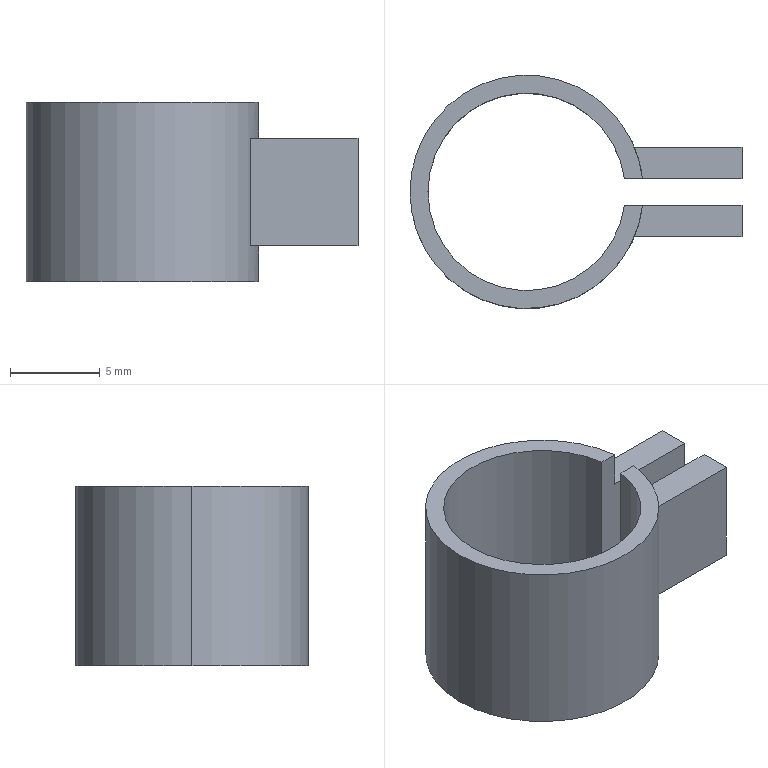Part | SolidWorks | features ICE 2, ExtruThin 1 | 1 solid | 16 faces | box 18.5 x 13 x 10 mm | volume 482.242 mm3 | plane 12 | cylinder 4 | commonest cylinder face diameters 11 x2 13 x2
STEP:
#1=CARTESIAN_POINT('',(5.449,0.75,5.));
#2=VERTEX_POINT('',#1);
#3=CARTESIAN_POINT('',(-5.5,0.,5.));
#4=VERTEX_POINT('',#3);
#5=CARTESIAN_POINT('',(0.,0.,5.));
#6=DIRECTION('',(0.,0.,1.));
#7=DIRECTION('',(1.,0.,0.));
#8=AXIS2_PLACEMENT_3D('',#5,#6,#7);
#9=CIRCLE('',#8,5.5);
#10=EDGE_CURVE('',#2,#4,#9,.T.);
#11=ORIENTED_EDGE('',*,*,#10,.T.);
#12=CARTESIAN_POINT('',(-5.5,0.,-5.));
#13=VERTEX_POINT('',#12);
#14=CARTESIAN_POINT('',(-5.5,0.,5.));
#15=DIRECTION('',(0.,0.,-1.));
#16=VECTOR('',#15,1000.);
#17=LINE('',#14,#16);
#18=EDGE_CURVE('',#4,#13,#17,.T.);
#19=ORIENTED_EDGE('',*,*,#18,.T.);
#20=CARTESIAN_POINT('',(5.449,0.75,-5.));
#21=VERTEX_POINT('',#20);
#22=CARTESIAN_POINT('',(0.,0.,-5.));
#23=DIRECTION('',(0.,0.,1.));
#24=DIRECTION('',(1.,0.,0.));
#25=AXIS2_PLACEMENT_3D('',#22,#23,#24);
#26=CIRCLE('',#25,5.5);
#27=EDGE_CURVE('',#21,#13,#26,.T.);
#28=ORIENTED_EDGE('',*,*,#27,.F.);
#29=CARTESIAN_POINT('',(5.449,0.75,5.));
#30=DIRECTION('',(0.,0.,-1.));
#31=VECTOR('',#30,1000.);
#32=LINE('',#29,#31);
#33=EDGE_CURVE('',#2,#21,#32,.T.);
#34=ORIENTED_EDGE('',*,*,#33,.F.);
#35=EDGE_LOOP('',(#11,#19,#28,#34));
#36=FACE_OUTER_BOUND('',#35,.T.);
#37=CARTESIAN_POINT('',(0.,0.,5.));
#38=DIRECTION('',(0.,0.,-1.));
#39=DIRECTION('',(-1.,0.,0.));
#40=AXIS2_PLACEMENT_3D('',#37,#38,#39);
#41=CYLINDRICAL_SURFACE('',#40,5.5);
#42=ADVANCED_FACE('',(#36),#41,.F.);
#43=CARTESIAN_POINT('',(-6.5,0.,5.));
#44=VERTEX_POINT('',#43);
#45=CARTESIAN_POINT('',(6.457,-0.75,5.));
#46=VERTEX_POINT('',#45);
#47=CARTESIAN_POINT('',(0.,0.,5.));
#48=DIRECTION('',(0.,0.,1.));
#49=DIRECTION('',(1.,0.,0.));
#50=AXIS2_PLACEMENT_3D('',#47,#48,#49);
#51=CIRCLE('',#50,6.5);
#52=EDGE_CURVE('',#44,#46,#51,.T.);
#53=ORIENTED_EDGE('',*,*,#52,.F.);
#54=CARTESIAN_POINT('',(-6.5,0.,-5.));
#55=VERTEX_POINT('',#54);
#56=CARTESIAN_POINT('',(-6.5,0.,5.));
#57=DIRECTION('',(0.,0.,-1.));
#58=VECTOR('',#57,1000.);
#59=LINE('',#56,#58);
#60=EDGE_CURVE('',#44,#55,#59,.T.);
#61=ORIENTED_EDGE('',*,*,#60,.T.);
#62=CARTESIAN_POINT('',(6.457,-0.75,-5.));
#63=VERTEX_POINT('',#62);
#64=CARTESIAN_POINT('',(0.,0.,-5.));
#65=DIRECTION('',(0.,0.,1.));
#66=DIRECTION('',(1.,0.,0.));
#67=AXIS2_PLACEMENT_3D('',#64,#65,#66);
#68=CIRCLE('',#67,6.5);
#69=EDGE_CURVE('',#55,#63,#68,.T.);
#70=ORIENTED_EDGE('',*,*,#69,.T.);
#71=CARTESIAN_POINT('',(6.457,-0.75,-3.));
#72=VERTEX_POINT('',#71);
#73=CARTESIAN_POINT('',(6.457,-0.75,5.));
#74=DIRECTION('',(0.,0.,1.));
#75=VECTOR('',#74,1000.);
#76=LINE('',#73,#75);
#77=EDGE_CURVE('',#63,#72,#76,.T.);
#78=ORIENTED_EDGE('',*,*,#77,.T.);
#79=CARTESIAN_POINT('',(6.,-2.5,-3.));
#80=VERTEX_POINT('',#79);
#81=CARTESIAN_POINT('',(0.,0.,-3.));
#82=DIRECTION('',(0.,0.,1.));
#83=DIRECTION('',(1.,0.,0.));
#84=AXIS2_PLACEMENT_3D('',#81,#82,#83);
#85=CIRCLE('',#84,6.5);
#86=EDGE_CURVE('',#80,#72,#85,.T.);
#87=ORIENTED_EDGE('',*,*,#86,.F.);
#88=CARTESIAN_POINT('',(6.,-2.5,3.));
#89=VERTEX_POINT('',#88);
#90=CARTESIAN_POINT('',(6.,-2.5,3.));
#91=DIRECTION('',(0.,0.,-1.));
#92=VECTOR('',#91,1000.);
#93=LINE('',#90,#92);
#94=EDGE_CURVE('',#89,#80,#93,.T.);
#95=ORIENTED_EDGE('',*,*,#94,.F.);
#96=CARTESIAN_POINT('',(6.457,-0.75,3.));
#97=VERTEX_POINT('',#96);
#98=CARTESIAN_POINT('',(0.,0.,3.));
#99=DIRECTION('',(0.,0.,1.));
#100=DIRECTION('',(1.,0.,0.));
#101=AXIS2_PLACEMENT_3D('',#98,#99,#100);
#102=CIRCLE('',#101,6.5);
#103=EDGE_CURVE('',#89,#97,#102,.T.);
#104=ORIENTED_EDGE('',*,*,#103,.T.);
#105=CARTESIAN_POINT('',(6.457,-0.75,5.));
#106=DIRECTION('',(0.,0.,1.));
#107=VECTOR('',#106,1000.);
#108=LINE('',#105,#107);
#109=EDGE_CURVE('',#97,#46,#108,.T.);
#110=ORIENTED_EDGE('',*,*,#109,.T.);
#111=EDGE_LOOP('',(#53,#61,#70,#78,#87,#95,#104,#110));
#112=FACE_OUTER_BOUND('',#111,.T.);
#113=CARTESIAN_POINT('',(0.,0.,5.));
#114=DIRECTION('',(0.,0.,-1.));
#115=DIRECTION('',(-1.,0.,0.));
#116=AXIS2_PLACEMENT_3D('',#113,#114,#115);
#117=CYLINDRICAL_SURFACE('',#116,6.5);
#118=ADVANCED_FACE('',(#112),#117,.T.);
#119=CARTESIAN_POINT('',(12.,0.75,3.));
#120=VERTEX_POINT('',#119);
#121=CARTESIAN_POINT('',(12.,2.5,3.));
#122=VERTEX_POINT('',#121);
#123=CARTESIAN_POINT('',(12.,2.5,3.));
#124=DIRECTION('',(0.,1.,0.));
#125=VECTOR('',#124,1000.);
#126=LINE('',#123,#125);
#127=EDGE_CURVE('',#120,#122,#126,.T.);
#128=ORIENTED_EDGE('',*,*,#127,.F.);
#129=CARTESIAN_POINT('',(12.,0.75,-3.));
#130=VERTEX_POINT('',#129);
#131=CARTESIAN_POINT('',(12.,0.75,3.));
#132=DIRECTION('',(0.,0.,-1.));
#133=VECTOR('',#132,1000.);
#134=LINE('',#131,#133);
#135=EDGE_CURVE('',#120,#130,#134,.T.);
#136=ORIENTED_EDGE('',*,*,#135,.T.);
#137=CARTESIAN_POINT('',(12.,2.5,-3.));
#138=VERTEX_POINT('',#137);
#139=CARTESIAN_POINT('',(12.,2.5,-3.));
#140=DIRECTION('',(0.,1.,0.));
#141=VECTOR('',#140,1000.);
#142=LINE('',#139,#141);
#143=EDGE_CURVE('',#130,#138,#142,.T.);
#144=ORIENTED_EDGE('',*,*,#143,.T.);
#145=CARTESIAN_POINT('',(12.,2.5,3.));
#146=DIRECTION('',(0.,0.,-1.));
#147=VECTOR('',#146,1000.);
#148=LINE('',#145,#147);
#149=EDGE_CURVE('',#122,#138,#148,.T.);
#150=ORIENTED_EDGE('',*,*,#149,.F.);
#151=EDGE_LOOP('',(#128,#136,#144,#150));
#152=FACE_OUTER_BOUND('',#151,.T.);
#153=CARTESIAN_POINT('',(12.,2.5,3.));
#154=DIRECTION('',(-1.,0.,0.));
#155=DIRECTION('',(0.,0.,1.));
#156=AXIS2_PLACEMENT_3D('',#153,#154,#155);
#157=PLANE('',#156);
#158=ADVANCED_FACE('',(#152),#157,.F.);
#159=CARTESIAN_POINT('',(6.457,0.75,3.));
#160=VERTEX_POINT('',#159);
#161=CARTESIAN_POINT('',(0.,0.75,3.));
#162=DIRECTION('',(-1.,0.,0.));
#163=VECTOR('',#162,1000.);
#164=LINE('',#161,#163);
#165=EDGE_CURVE('',#120,#160,#164,.T.);
#166=ORIENTED_EDGE('',*,*,#165,.F.);
#167=ORIENTED_EDGE('',*,*,#127,.T.);
#168=CARTESIAN_POINT('',(6.,2.5,3.));
#169=VERTEX_POINT('',#168);
#170=CARTESIAN_POINT('',(6.,2.5,3.));
#171=DIRECTION('',(-1.,0.,0.));
#172=VECTOR('',#171,1000.);
#173=LINE('',#170,#172);
#174=EDGE_CURVE('',#122,#169,#173,.T.);
#175=ORIENTED_EDGE('',*,*,#174,.T.);
#176=CARTESIAN_POINT('',(0.,0.,3.));
#177=DIRECTION('',(0.,0.,1.));
#178=DIRECTION('',(1.,0.,0.));
#179=AXIS2_PLACEMENT_3D('',#176,#177,#178);
#180=CIRCLE('',#179,6.5);
#181=EDGE_CURVE('',#160,#169,#180,.T.);
#182=ORIENTED_EDGE('',*,*,#181,.F.);
#183=EDGE_LOOP('',(#166,#167,#175,#182));
#184=FACE_OUTER_BOUND('',#183,.T.);
#185=CARTESIAN_POINT('',(0.,0.,3.));
#186=DIRECTION('',(0.,0.,1.));
#187=DIRECTION('',(1.,0.,0.));
#188=AXIS2_PLACEMENT_3D('',#185,#186,#187);
#189=PLANE('',#188);
#190=ADVANCED_FACE('',(#184),#189,.T.);
#191=ORIENTED_EDGE('',*,*,#143,.F.);
#192=CARTESIAN_POINT('',(6.457,0.75,-3.));
#193=VERTEX_POINT('',#192);
#194=CARTESIAN_POINT('',(0.,0.75,-3.));
#195=DIRECTION('',(-1.,0.,0.));
#196=VECTOR('',#195,1000.);
#197=LINE('',#194,#196);
#198=EDGE_CURVE('',#130,#193,#197,.T.);
#199=ORIENTED_EDGE('',*,*,#198,.T.);
#200=CARTESIAN_POINT('',(6.,2.5,-3.));
#201=VERTEX_POINT('',#200);
#202=CARTESIAN_POINT('',(0.,0.,-3.));
#203=DIRECTION('',(0.,0.,1.));
#204=DIRECTION('',(1.,0.,0.));
#205=AXIS2_PLACEMENT_3D('',#202,#203,#204);
#206=CIRCLE('',#205,6.5);
#207=EDGE_CURVE('',#193,#201,#206,.T.);
#208=ORIENTED_EDGE('',*,*,#207,.T.);
#209=CARTESIAN_POINT('',(6.,2.5,-3.));
#210=DIRECTION('',(-1.,0.,0.));
#211=VECTOR('',#210,1000.);
#212=LINE('',#209,#211);
#213=EDGE_CURVE('',#138,#201,#212,.T.);
#214=ORIENTED_EDGE('',*,*,#213,.F.);
#215=EDGE_LOOP('',(#191,#199,#208,#214));
#216=FACE_OUTER_BOUND('',#215,.T.);
#217=CARTESIAN_POINT('',(0.,0.,-3.));
#218=DIRECTION('',(0.,0.,1.));
#219=DIRECTION('',(1.,0.,0.));
#220=AXIS2_PLACEMENT_3D('',#217,#218,#219);
#221=PLANE('',#220);
#222=ADVANCED_FACE('',(#216),#221,.F.);
#223=CARTESIAN_POINT('',(6.457,0.75,5.));
#224=VERTEX_POINT('',#223);
#225=CARTESIAN_POINT('',(0.,0.75,5.));
#226=DIRECTION('',(-1.,0.,0.));
#227=VECTOR('',#226,1000.);
#228=LINE('',#225,#227);
#229=EDGE_CURVE('',#224,#2,#228,.T.);
#230=ORIENTED_EDGE('',*,*,#229,.F.);
#231=CARTESIAN_POINT('',(0.,0.,5.));
#232=DIRECTION('',(0.,0.,1.));
#233=DIRECTION('',(1.,0.,0.));
#234=AXIS2_PLACEMENT_3D('',#231,#232,#233);
#235=CIRCLE('',#234,6.5);
#236=EDGE_CURVE('',#224,#44,#235,.T.);
#237=ORIENTED_EDGE('',*,*,#236,.T.);
#238=ORIENTED_EDGE('',*,*,#52,.T.);
#239=CARTESIAN_POINT('',(5.449,-0.75,5.));
#240=VERTEX_POINT('',#239);
#241=CARTESIAN_POINT('',(0.,-0.75,5.));
#242=DIRECTION('',(1.,0.,0.));
#243=VECTOR('',#242,1000.);
#244=LINE('',#241,#243);
#245=EDGE_CURVE('',#240,#46,#244,.T.);
#246=ORIENTED_EDGE('',*,*,#245,.F.);
#247=CARTESIAN_POINT('',(0.,0.,5.));
#248=DIRECTION('',(0.,0.,1.));
#249=DIRECTION('',(1.,0.,0.));
#250=AXIS2_PLACEMENT_3D('',#247,#248,#249);
#251=CIRCLE('',#250,5.5);
#252=EDGE_CURVE('',#4,#240,#251,.T.);
#253=ORIENTED_EDGE('',*,*,#252,.F.);
#254=ORIENTED_EDGE('',*,*,#10,.F.);
#255=EDGE_LOOP('',(#230,#237,#238,#246,#253,#254));
#256=FACE_OUTER_BOUND('',#255,.T.);
#257=CARTESIAN_POINT('',(0.,0.,5.));
#258=DIRECTION('',(0.,0.,1.));
#259=DIRECTION('',(1.,0.,0.));
#260=AXIS2_PLACEMENT_3D('',#257,#258,#259);
#261=PLANE('',#260);
#262=ADVANCED_FACE('',(#256),#261,.T.);
#263=CARTESIAN_POINT('',(6.457,0.75,-5.));
#264=VERTEX_POINT('',#263);
#265=CARTESIAN_POINT('',(0.,0.,-5.));
#266=DIRECTION('',(0.,0.,1.));
#267=DIRECTION('',(1.,0.,0.));
#268=AXIS2_PLACEMENT_3D('',#265,#266,#267);
#269=CIRCLE('',#268,6.5);
#270=EDGE_CURVE('',#264,#55,#269,.T.);
#271=ORIENTED_EDGE('',*,*,#270,.F.);
#272=CARTESIAN_POINT('',(0.,0.75,-5.));
#273=DIRECTION('',(-1.,0.,0.));
#274=VECTOR('',#273,1000.);
#275=LINE('',#272,#274);
#276=EDGE_CURVE('',#264,#21,#275,.T.);
#277=ORIENTED_EDGE('',*,*,#276,.T.);
#278=ORIENTED_EDGE('',*,*,#27,.T.);
#279=CARTESIAN_POINT('',(5.449,-0.75,-5.));
#280=VERTEX_POINT('',#279);
#281=CARTESIAN_POINT('',(0.,0.,-5.));
#282=DIRECTION('',(0.,0.,1.));
#283=DIRECTION('',(1.,0.,0.));
#284=AXIS2_PLACEMENT_3D('',#281,#282,#283);
#285=CIRCLE('',#284,5.5);
#286=EDGE_CURVE('',#13,#280,#285,.T.);
#287=ORIENTED_EDGE('',*,*,#286,.T.);
#288=CARTESIAN_POINT('',(0.,-0.75,-5.));
#289=DIRECTION('',(1.,0.,0.));
#290=VECTOR('',#289,1000.);
#291=LINE('',#288,#290);
#292=EDGE_CURVE('',#280,#63,#291,.T.);
#293=ORIENTED_EDGE('',*,*,#292,.T.);
#294=ORIENTED_EDGE('',*,*,#69,.F.);
#295=EDGE_LOOP('',(#271,#277,#278,#287,#293,#294));
#296=FACE_OUTER_BOUND('',#295,.T.);
#297=CARTESIAN_POINT('',(0.,0.,-5.));
#298=DIRECTION('',(0.,0.,1.));
#299=DIRECTION('',(1.,0.,0.));
#300=AXIS2_PLACEMENT_3D('',#297,#298,#299);
#301=PLANE('',#300);
#302=ADVANCED_FACE('',(#296),#301,.F.);
#303=ORIENTED_EDGE('',*,*,#60,.F.);
#304=ORIENTED_EDGE('',*,*,#236,.F.);
#305=CARTESIAN_POINT('',(6.457,0.75,5.));
#306=DIRECTION('',(0.,0.,-1.));
#307=VECTOR('',#306,1000.);
#308=LINE('',#305,#307);
#309=EDGE_CURVE('',#224,#160,#308,.T.);
#310=ORIENTED_EDGE('',*,*,#309,.T.);
#311=ORIENTED_EDGE('',*,*,#181,.T.);
#312=CARTESIAN_POINT('',(6.,2.5,3.));
#313=DIRECTION('',(0.,0.,-1.));
#314=VECTOR('',#313,1000.);
#315=LINE('',#312,#314);
#316=EDGE_CURVE('',#169,#201,#315,.T.);
#317=ORIENTED_EDGE('',*,*,#316,.T.);
#318=ORIENTED_EDGE('',*,*,#207,.F.);
#319=CARTESIAN_POINT('',(6.457,0.75,5.));
#320=DIRECTION('',(0.,0.,-1.));
#321=VECTOR('',#320,1000.);
#322=LINE('',#319,#321);
#323=EDGE_CURVE('',#193,#264,#322,.T.);
#324=ORIENTED_EDGE('',*,*,#323,.T.);
#325=ORIENTED_EDGE('',*,*,#270,.T.);
#326=EDGE_LOOP('',(#303,#304,#310,#311,#317,#318,#324,#325));
#327=FACE_OUTER_BOUND('',#326,.T.);
#328=CARTESIAN_POINT('',(0.,0.,5.));
#329=DIRECTION('',(0.,0.,-1.));
#330=DIRECTION('',(-1.,0.,0.));
#331=AXIS2_PLACEMENT_3D('',#328,#329,#330);
#332=CYLINDRICAL_SURFACE('',#331,6.5);
#333=ADVANCED_FACE('',(#327),#332,.T.);
#334=ORIENTED_EDGE('',*,*,#18,.F.);
#335=ORIENTED_EDGE('',*,*,#252,.T.);
#336=CARTESIAN_POINT('',(5.449,-0.75,5.));
#337=DIRECTION('',(0.,0.,1.));
#338=VECTOR('',#337,1000.);
#339=LINE('',#336,#338);
#340=EDGE_CURVE('',#280,#240,#339,.T.);
#341=ORIENTED_EDGE('',*,*,#340,.F.);
#342=ORIENTED_EDGE('',*,*,#286,.F.);
#343=EDGE_LOOP('',(#334,#335,#341,#342));
#344=FACE_OUTER_BOUND('',#343,.T.);
#345=CARTESIAN_POINT('',(0.,0.,5.));
#346=DIRECTION('',(0.,0.,-1.));
#347=DIRECTION('',(-1.,0.,0.));
#348=AXIS2_PLACEMENT_3D('',#345,#346,#347);
#349=CYLINDRICAL_SURFACE('',#348,5.5);
#350=ADVANCED_FACE('',(#344),#349,.F.);
#351=CARTESIAN_POINT('',(12.,-2.5,-3.));
#352=VERTEX_POINT('',#351);
#353=CARTESIAN_POINT('',(6.,-2.5,-3.));
#354=DIRECTION('',(1.,0.,0.));
#355=VECTOR('',#354,1000.);
#356=LINE('',#353,#355);
#357=EDGE_CURVE('',#80,#352,#356,.T.);
#358=ORIENTED_EDGE('',*,*,#357,.T.);
#359=CARTESIAN_POINT('',(12.,-2.5,3.));
#360=VERTEX_POINT('',#359);
#361=CARTESIAN_POINT('',(12.,-2.5,3.));
#362=DIRECTION('',(0.,0.,-1.));
#363=VECTOR('',#362,1000.);
#364=LINE('',#361,#363);
#365=EDGE_CURVE('',#360,#352,#364,.T.);
#366=ORIENTED_EDGE('',*,*,#365,.F.);
#367=CARTESIAN_POINT('',(6.,-2.5,3.));
#368=DIRECTION('',(1.,0.,0.));
#369=VECTOR('',#368,1000.);
#370=LINE('',#367,#369);
#371=EDGE_CURVE('',#89,#360,#370,.T.);
#372=ORIENTED_EDGE('',*,*,#371,.F.);
#373=ORIENTED_EDGE('',*,*,#94,.T.);
#374=EDGE_LOOP('',(#358,#366,#372,#373));
#375=FACE_OUTER_BOUND('',#374,.T.);
#376=CARTESIAN_POINT('',(6.,-2.5,3.));
#377=DIRECTION('',(0.,1.,0.));
#378=DIRECTION('',(0.,0.,1.));
#379=AXIS2_PLACEMENT_3D('',#376,#377,#378);
#380=PLANE('',#379);
#381=ADVANCED_FACE('',(#375),#380,.F.);
#382=CARTESIAN_POINT('',(12.,-0.75,-3.));
#383=VERTEX_POINT('',#382);
#384=CARTESIAN_POINT('',(12.,2.5,-3.));
#385=DIRECTION('',(0.,1.,0.));
#386=VECTOR('',#385,1000.);
#387=LINE('',#384,#386);
#388=EDGE_CURVE('',#352,#383,#387,.T.);
#389=ORIENTED_EDGE('',*,*,#388,.T.);
#390=CARTESIAN_POINT('',(12.,-0.75,3.));
#391=VERTEX_POINT('',#390);
#392=CARTESIAN_POINT('',(12.,-0.75,3.));
#393=DIRECTION('',(0.,0.,1.));
#394=VECTOR('',#393,1000.);
#395=LINE('',#392,#394);
#396=EDGE_CURVE('',#383,#391,#395,.T.);
#397=ORIENTED_EDGE('',*,*,#396,.T.);
#398=CARTESIAN_POINT('',(12.,2.5,3.));
#399=DIRECTION('',(0.,1.,0.));
#400=VECTOR('',#399,1000.);
#401=LINE('',#398,#400);
#402=EDGE_CURVE('',#360,#391,#401,.T.);
#403=ORIENTED_EDGE('',*,*,#402,.F.);
#404=ORIENTED_EDGE('',*,*,#365,.T.);
#405=EDGE_LOOP('',(#389,#397,#403,#404));
#406=FACE_OUTER_BOUND('',#405,.T.);
#407=CARTESIAN_POINT('',(12.,2.5,3.));
#408=DIRECTION('',(-1.,0.,0.));
#409=DIRECTION('',(0.,0.,1.));
#410=AXIS2_PLACEMENT_3D('',#407,#408,#409);
#411=PLANE('',#410);
#412=ADVANCED_FACE('',(#406),#411,.F.);
#413=ORIENTED_EDGE('',*,*,#213,.T.);
#414=ORIENTED_EDGE('',*,*,#316,.F.);
#415=ORIENTED_EDGE('',*,*,#174,.F.);
#416=ORIENTED_EDGE('',*,*,#149,.T.);
#417=EDGE_LOOP('',(#413,#414,#415,#416));
#418=FACE_OUTER_BOUND('',#417,.T.);
#419=CARTESIAN_POINT('',(6.,2.5,3.));
#420=DIRECTION('',(0.,-1.,0.));
#421=DIRECTION('',(0.,0.,-1.));
#422=AXIS2_PLACEMENT_3D('',#419,#420,#421);
#423=PLANE('',#422);
#424=ADVANCED_FACE('',(#418),#423,.F.);
#425=CARTESIAN_POINT('',(0.,-0.75,3.));
#426=DIRECTION('',(1.,0.,0.));
#427=VECTOR('',#426,1000.);
#428=LINE('',#425,#427);
#429=EDGE_CURVE('',#97,#391,#428,.T.);
#430=ORIENTED_EDGE('',*,*,#429,.F.);
#431=ORIENTED_EDGE('',*,*,#103,.F.);
#432=ORIENTED_EDGE('',*,*,#371,.T.);
#433=ORIENTED_EDGE('',*,*,#402,.T.);
#434=EDGE_LOOP('',(#430,#431,#432,#433));
#435=FACE_OUTER_BOUND('',#434,.T.);
#436=CARTESIAN_POINT('',(0.,0.,3.));
#437=DIRECTION('',(0.,0.,1.));
#438=DIRECTION('',(1.,0.,0.));
#439=AXIS2_PLACEMENT_3D('',#436,#437,#438);
#440=PLANE('',#439);
#441=ADVANCED_FACE('',(#435),#440,.T.);
#442=ORIENTED_EDGE('',*,*,#86,.T.);
#443=CARTESIAN_POINT('',(0.,-0.75,-3.));
#444=DIRECTION('',(1.,0.,0.));
#445=VECTOR('',#444,1000.);
#446=LINE('',#443,#445);
#447=EDGE_CURVE('',#72,#383,#446,.T.);
#448=ORIENTED_EDGE('',*,*,#447,.T.);
#449=ORIENTED_EDGE('',*,*,#388,.F.);
#450=ORIENTED_EDGE('',*,*,#357,.F.);
#451=EDGE_LOOP('',(#442,#448,#449,#450));
#452=FACE_OUTER_BOUND('',#451,.T.);
#453=CARTESIAN_POINT('',(0.,0.,-3.));
#454=DIRECTION('',(0.,0.,1.));
#455=DIRECTION('',(1.,0.,0.));
#456=AXIS2_PLACEMENT_3D('',#453,#454,#455);
#457=PLANE('',#456);
#458=ADVANCED_FACE('',(#452),#457,.F.);
#459=ORIENTED_EDGE('',*,*,#340,.T.);
#460=ORIENTED_EDGE('',*,*,#245,.T.);
#461=ORIENTED_EDGE('',*,*,#109,.F.);
#462=ORIENTED_EDGE('',*,*,#429,.T.);
#463=ORIENTED_EDGE('',*,*,#396,.F.);
#464=ORIENTED_EDGE('',*,*,#447,.F.);
#465=ORIENTED_EDGE('',*,*,#77,.F.);
#466=ORIENTED_EDGE('',*,*,#292,.F.);
#467=EDGE_LOOP('',(#459,#460,#461,#462,#463,#464,#465,#466));
#468=FACE_OUTER_BOUND('',#467,.T.);
#469=CARTESIAN_POINT('',(0.,-0.75,-5.));
#470=DIRECTION('',(0.,-1.,0.));
#471=DIRECTION('',(0.,0.,-1.));
#472=AXIS2_PLACEMENT_3D('',#469,#470,#471);
#473=PLANE('',#472);
#474=ADVANCED_FACE('',(#468),#473,.F.);
#475=ORIENTED_EDGE('',*,*,#33,.T.);
#476=ORIENTED_EDGE('',*,*,#276,.F.);
#477=ORIENTED_EDGE('',*,*,#323,.F.);
#478=ORIENTED_EDGE('',*,*,#198,.F.);
#479=ORIENTED_EDGE('',*,*,#135,.F.);
#480=ORIENTED_EDGE('',*,*,#165,.T.);
#481=ORIENTED_EDGE('',*,*,#309,.F.);
#482=ORIENTED_EDGE('',*,*,#229,.T.);
#483=EDGE_LOOP('',(#475,#476,#477,#478,#479,#480,#481,#482));
#484=FACE_OUTER_BOUND('',#483,.T.);
#485=CARTESIAN_POINT('',(0.,0.75,-5.));
#486=DIRECTION('',(0.,1.,0.));
#487=DIRECTION('',(0.,0.,1.));
#488=AXIS2_PLACEMENT_3D('',#485,#486,#487);
#489=PLANE('',#488);
#490=ADVANCED_FACE('',(#484),#489,.F.);
#491=CLOSED_SHELL('',(#42,#118,#158,#190,#222,#262,#302,#333,#350,#381,#412,#424,#441,#458,#474,#490));
#492=MANIFOLD_SOLID_BREP('',#491);
#493=CARTESIAN_POINT('',(0.,0.,0.));
#494=DIRECTION('',(0.,0.,1.));
#495=DIRECTION('',(1.,0.,0.));
#496=AXIS2_PLACEMENT_3D('',#493,#494,#495);
#497=(LENGTH_UNIT()NAMED_UNIT(*)SI_UNIT(.MILLI.,.METRE.));
#498=UNCERTAINTY_MEASURE_WITH_UNIT(LENGTH_MEASURE(0.00001),#497,'','');
#499=(NAMED_UNIT(*)PLANE_ANGLE_UNIT()SI_UNIT($,.RADIAN.));
#500=(NAMED_UNIT(*)SI_UNIT($,.STERADIAN.)SOLID_ANGLE_UNIT());
#501=(GEOMETRIC_REPRESENTATION_CONTEXT(3)GLOBAL_UNCERTAINTY_ASSIGNED_CONTEXT((#498))GLOBAL_UNIT_ASSIGNED_CONTEXT((#497,#499,#500))REPRESENTATION_CONTEXT('',''));
#502=ADVANCED_BREP_SHAPE_REPRESENTATION('',(#492,#496),#501);